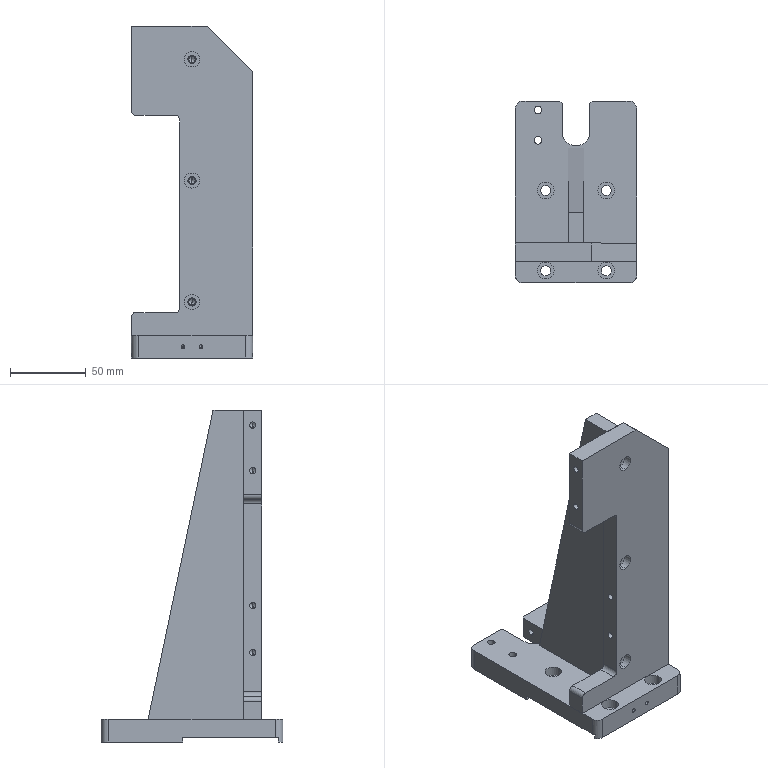Part | STEP file | PN_0013 | 3 solids | 214 faces | box 80 x 120 x 219 mm | volume 332786 mm3 | cylinder 125 | plane 55 | cone 34 | commonest cylinder face diameters 5.5 x36 4.2 x28 10 x24 4 x8 6.6 x8 11 x8